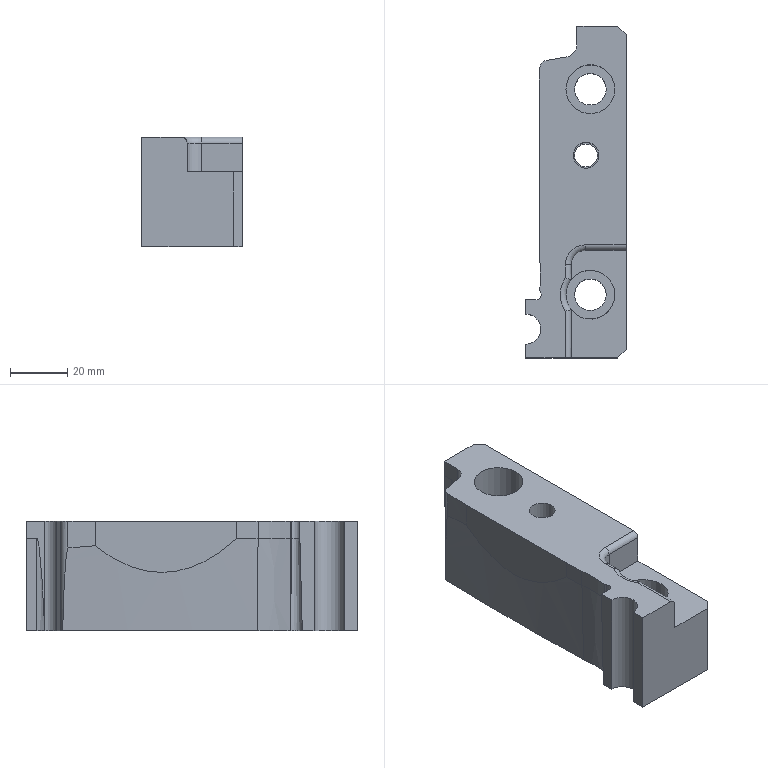Part | STEP file | 1_id110_x_t | 1 solid | 47 faces | box 35 x 115.5 x 38.1 mm | volume 106763 mm3 | plane 22 | cylinder 18 | cone 5 | torus 2 | commonest cylinder face diameters 4 x3 11 x2 17 x2 2204 x2 2.4 x1 3.6 x1